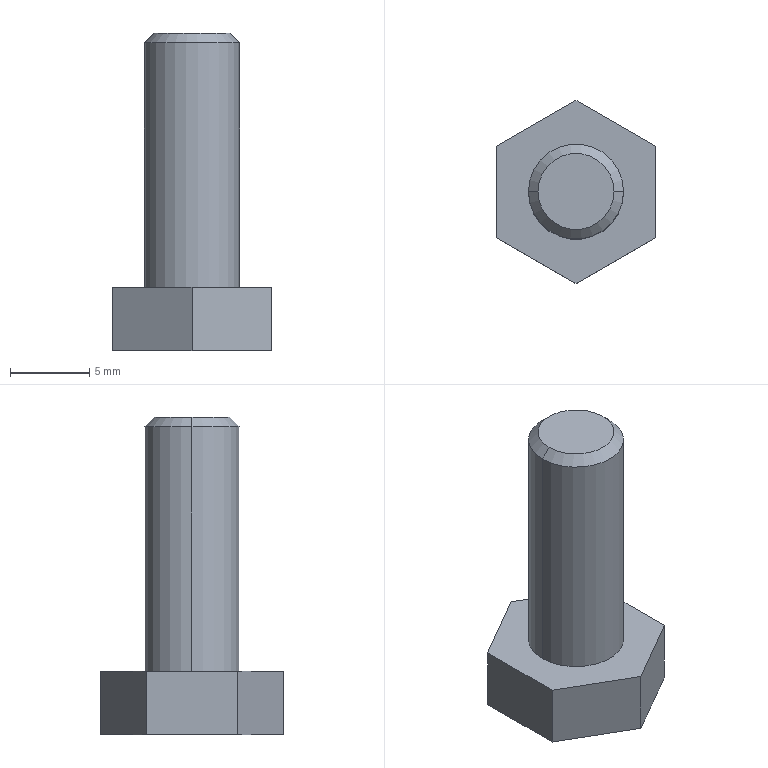Part | SolidWorks | features Chamfer 1, Extrusion 1, ICE 1, RefAxis 1 | 1 solid | 13 faces | box 10 x 11.547 x 20 mm | volume 795.633 mm3 | plane 9 | cone 2 | cylinder 2 | commonest cylinder face diameters 6 x2
STEP:
#1=CARTESIAN_POINT('',(2.4,0.,20.));
#2=VERTEX_POINT('',#1);
#3=CARTESIAN_POINT('',(-2.4,0.,20.));
#4=VERTEX_POINT('',#3);
#5=CARTESIAN_POINT('',(0.,0.,20.));
#6=DIRECTION('',(0.,0.,1.));
#7=DIRECTION('',(1.,0.,0.));
#8=AXIS2_PLACEMENT_3D('',#5,#6,#7);
#9=CIRCLE('',#8,2.4);
#10=EDGE_CURVE('',#2,#4,#9,.T.);
#11=ORIENTED_EDGE('',*,*,#10,.F.);
#12=CARTESIAN_POINT('',(3.,0.,19.4));
#13=VERTEX_POINT('',#12);
#14=CARTESIAN_POINT('',(2.4,0.,20.));
#15=DIRECTION('',(0.7071,0.,-0.7071));
#16=VECTOR('',#15,1000.);
#17=LINE('',#14,#16);
#18=EDGE_CURVE('',#2,#13,#17,.T.);
#19=ORIENTED_EDGE('',*,*,#18,.T.);
#20=CARTESIAN_POINT('',(-3.,0.,19.4));
#21=VERTEX_POINT('',#20);
#22=CARTESIAN_POINT('',(0.,0.,19.4));
#23=DIRECTION('',(0.,0.,-1.));
#24=DIRECTION('',(1.,0.,0.));
#25=AXIS2_PLACEMENT_3D('',#22,#23,#24);
#26=CIRCLE('',#25,3.);
#27=EDGE_CURVE('',#21,#13,#26,.T.);
#28=ORIENTED_EDGE('',*,*,#27,.F.);
#29=CARTESIAN_POINT('',(-2.4,0.,20.));
#30=DIRECTION('',(-0.7071,0.,-0.7071));
#31=VECTOR('',#30,1000.);
#32=LINE('',#29,#31);
#33=EDGE_CURVE('',#4,#21,#32,.T.);
#34=ORIENTED_EDGE('',*,*,#33,.F.);
#35=EDGE_LOOP('',(#11,#19,#28,#34));
#36=FACE_OUTER_BOUND('',#35,.T.);
#37=CARTESIAN_POINT('',(0.,0.,20.));
#38=DIRECTION('',(0.,0.,-1.));
#39=DIRECTION('',(-1.,0.,0.));
#40=AXIS2_PLACEMENT_3D('',#37,#38,#39);
#41=CONICAL_SURFACE('',#40,2.4,0.7854);
#42=ADVANCED_FACE('',(#36),#41,.T.);
#43=ORIENTED_EDGE('',*,*,#27,.T.);
#44=CARTESIAN_POINT('',(3.,0.,4.));
#45=VERTEX_POINT('',#44);
#46=CARTESIAN_POINT('',(3.,0.,20.));
#47=DIRECTION('',(0.,0.,-1.));
#48=VECTOR('',#47,1000.);
#49=LINE('',#46,#48);
#50=EDGE_CURVE('',#13,#45,#49,.T.);
#51=ORIENTED_EDGE('',*,*,#50,.T.);
#52=CARTESIAN_POINT('',(-3.,0.,4.));
#53=VERTEX_POINT('',#52);
#54=CARTESIAN_POINT('',(0.,0.,4.));
#55=DIRECTION('',(0.,0.,1.));
#56=DIRECTION('',(1.,0.,0.));
#57=AXIS2_PLACEMENT_3D('',#54,#55,#56);
#58=CIRCLE('',#57,3.);
#59=EDGE_CURVE('',#45,#53,#58,.T.);
#60=ORIENTED_EDGE('',*,*,#59,.T.);
#61=CARTESIAN_POINT('',(-3.,0.,20.));
#62=DIRECTION('',(0.,0.,-1.));
#63=VECTOR('',#62,1000.);
#64=LINE('',#61,#63);
#65=EDGE_CURVE('',#21,#53,#64,.T.);
#66=ORIENTED_EDGE('',*,*,#65,.F.);
#67=EDGE_LOOP('',(#43,#51,#60,#66));
#68=FACE_OUTER_BOUND('',#67,.T.);
#69=CARTESIAN_POINT('',(0.,0.,20.));
#70=DIRECTION('',(0.,0.,-1.));
#71=DIRECTION('',(-1.,0.,0.));
#72=AXIS2_PLACEMENT_3D('',#69,#70,#71);
#73=CYLINDRICAL_SURFACE('',#72,3.);
#74=ADVANCED_FACE('',(#68),#73,.T.);
#75=CARTESIAN_POINT('',(5.,-2.887,4.));
#76=VERTEX_POINT('',#75);
#77=CARTESIAN_POINT('',(5.,2.887,4.));
#78=VERTEX_POINT('',#77);
#79=CARTESIAN_POINT('',(5.,-2.887,4.));
#80=DIRECTION('',(0.,1.,0.));
#81=VECTOR('',#80,1000.);
#82=LINE('',#79,#81);
#83=EDGE_CURVE('',#76,#78,#82,.T.);
#84=ORIENTED_EDGE('',*,*,#83,.T.);
#85=CARTESIAN_POINT('',(0.,5.774,4.));
#86=VERTEX_POINT('',#85);
#87=CARTESIAN_POINT('',(5.,2.887,4.));
#88=DIRECTION('',(-0.866,0.5,0.));
#89=VECTOR('',#88,1000.);
#90=LINE('',#87,#89);
#91=EDGE_CURVE('',#78,#86,#90,.T.);
#92=ORIENTED_EDGE('',*,*,#91,.T.);
#93=CARTESIAN_POINT('',(-5.,2.887,4.));
#94=VERTEX_POINT('',#93);
#95=CARTESIAN_POINT('',(0.,5.774,4.));
#96=DIRECTION('',(-0.866,-0.5,0.));
#97=VECTOR('',#96,1000.);
#98=LINE('',#95,#97);
#99=EDGE_CURVE('',#86,#94,#98,.T.);
#100=ORIENTED_EDGE('',*,*,#99,.T.);
#101=CARTESIAN_POINT('',(-5.,-2.887,4.));
#102=VERTEX_POINT('',#101);
#103=CARTESIAN_POINT('',(-5.,2.887,4.));
#104=DIRECTION('',(0.,-1.,0.));
#105=VECTOR('',#104,1000.);
#106=LINE('',#103,#105);
#107=EDGE_CURVE('',#94,#102,#106,.T.);
#108=ORIENTED_EDGE('',*,*,#107,.T.);
#109=CARTESIAN_POINT('',(0.,-5.774,4.));
#110=VERTEX_POINT('',#109);
#111=CARTESIAN_POINT('',(-5.,-2.887,4.));
#112=DIRECTION('',(0.866,-0.5,0.));
#113=VECTOR('',#112,1000.);
#114=LINE('',#111,#113);
#115=EDGE_CURVE('',#102,#110,#114,.T.);
#116=ORIENTED_EDGE('',*,*,#115,.T.);
#117=CARTESIAN_POINT('',(0.,-5.774,4.));
#118=DIRECTION('',(0.866,0.5,0.));
#119=VECTOR('',#118,1000.);
#120=LINE('',#117,#119);
#121=EDGE_CURVE('',#110,#76,#120,.T.);
#122=ORIENTED_EDGE('',*,*,#121,.T.);
#123=EDGE_LOOP('',(#84,#92,#100,#108,#116,#122));
#124=FACE_OUTER_BOUND('',#123,.T.);
#125=CARTESIAN_POINT('',(0.,0.,4.));
#126=DIRECTION('',(0.,0.,1.));
#127=DIRECTION('',(1.,0.,0.));
#128=AXIS2_PLACEMENT_3D('',#125,#126,#127);
#129=CIRCLE('',#128,3.);
#130=EDGE_CURVE('',#53,#45,#129,.T.);
#131=ORIENTED_EDGE('',*,*,#130,.F.);
#132=ORIENTED_EDGE('',*,*,#59,.F.);
#133=EDGE_LOOP('',(#131,#132));
#134=FACE_BOUND('',#133,.T.);
#135=CARTESIAN_POINT('',(0.,0.,4.));
#136=DIRECTION('',(0.,0.,1.));
#137=DIRECTION('',(1.,0.,0.));
#138=AXIS2_PLACEMENT_3D('',#135,#136,#137);
#139=PLANE('',#138);
#140=ADVANCED_FACE('',(#124,#134),#139,.T.);
#141=CARTESIAN_POINT('',(5.,-2.887,0.));
#142=VERTEX_POINT('',#141);
#143=CARTESIAN_POINT('',(5.,2.887,0.));
#144=VERTEX_POINT('',#143);
#145=CARTESIAN_POINT('',(5.,-2.887,0.));
#146=DIRECTION('',(0.,1.,0.));
#147=VECTOR('',#146,1000.);
#148=LINE('',#145,#147);
#149=EDGE_CURVE('',#142,#144,#148,.T.);
#150=ORIENTED_EDGE('',*,*,#149,.T.);
#151=CARTESIAN_POINT('',(5.,2.887,4.));
#152=DIRECTION('',(0.,0.,-1.));
#153=VECTOR('',#152,1000.);
#154=LINE('',#151,#153);
#155=EDGE_CURVE('',#78,#144,#154,.T.);
#156=ORIENTED_EDGE('',*,*,#155,.F.);
#157=ORIENTED_EDGE('',*,*,#83,.F.);
#158=CARTESIAN_POINT('',(5.,-2.887,4.));
#159=DIRECTION('',(0.,0.,-1.));
#160=VECTOR('',#159,1000.);
#161=LINE('',#158,#160);
#162=EDGE_CURVE('',#76,#142,#161,.T.);
#163=ORIENTED_EDGE('',*,*,#162,.T.);
#164=EDGE_LOOP('',(#150,#156,#157,#163));
#165=FACE_OUTER_BOUND('',#164,.T.);
#166=CARTESIAN_POINT('',(5.,-2.887,4.));
#167=DIRECTION('',(-1.,0.,0.));
#168=DIRECTION('',(0.,-1.,0.));
#169=AXIS2_PLACEMENT_3D('',#166,#167,#168);
#170=PLANE('',#169);
#171=ADVANCED_FACE('',(#165),#170,.F.);
#172=CARTESIAN_POINT('',(0.,5.774,0.));
#173=VERTEX_POINT('',#172);
#174=CARTESIAN_POINT('',(5.,2.887,0.));
#175=DIRECTION('',(-0.866,0.5,0.));
#176=VECTOR('',#175,1000.);
#177=LINE('',#174,#176);
#178=EDGE_CURVE('',#144,#173,#177,.T.);
#179=ORIENTED_EDGE('',*,*,#178,.T.);
#180=CARTESIAN_POINT('',(0.,5.774,4.));
#181=DIRECTION('',(0.,0.,-1.));
#182=VECTOR('',#181,1000.);
#183=LINE('',#180,#182);
#184=EDGE_CURVE('',#86,#173,#183,.T.);
#185=ORIENTED_EDGE('',*,*,#184,.F.);
#186=ORIENTED_EDGE('',*,*,#91,.F.);
#187=ORIENTED_EDGE('',*,*,#155,.T.);
#188=EDGE_LOOP('',(#179,#185,#186,#187));
#189=FACE_OUTER_BOUND('',#188,.T.);
#190=CARTESIAN_POINT('',(5.,2.887,4.));
#191=DIRECTION('',(-0.5,-0.866,0.));
#192=DIRECTION('',(0.866,-0.5,0.));
#193=AXIS2_PLACEMENT_3D('',#190,#191,#192);
#194=PLANE('',#193);
#195=ADVANCED_FACE('',(#189),#194,.F.);
#196=CARTESIAN_POINT('',(-5.,2.887,0.));
#197=VERTEX_POINT('',#196);
#198=CARTESIAN_POINT('',(0.,5.774,0.));
#199=DIRECTION('',(-0.866,-0.5,0.));
#200=VECTOR('',#199,1000.);
#201=LINE('',#198,#200);
#202=EDGE_CURVE('',#173,#197,#201,.T.);
#203=ORIENTED_EDGE('',*,*,#202,.T.);
#204=CARTESIAN_POINT('',(-5.,2.887,4.));
#205=DIRECTION('',(0.,0.,-1.));
#206=VECTOR('',#205,1000.);
#207=LINE('',#204,#206);
#208=EDGE_CURVE('',#94,#197,#207,.T.);
#209=ORIENTED_EDGE('',*,*,#208,.F.);
#210=ORIENTED_EDGE('',*,*,#99,.F.);
#211=ORIENTED_EDGE('',*,*,#184,.T.);
#212=EDGE_LOOP('',(#203,#209,#210,#211));
#213=FACE_OUTER_BOUND('',#212,.T.);
#214=CARTESIAN_POINT('',(0.,5.774,4.));
#215=DIRECTION('',(0.5,-0.866,0.));
#216=DIRECTION('',(0.866,0.5,0.));
#217=AXIS2_PLACEMENT_3D('',#214,#215,#216);
#218=PLANE('',#217);
#219=ADVANCED_FACE('',(#213),#218,.F.);
#220=CARTESIAN_POINT('',(-5.,-2.887,0.));
#221=VERTEX_POINT('',#220);
#222=CARTESIAN_POINT('',(-5.,2.887,0.));
#223=DIRECTION('',(0.,-1.,0.));
#224=VECTOR('',#223,1000.);
#225=LINE('',#222,#224);
#226=EDGE_CURVE('',#197,#221,#225,.T.);
#227=ORIENTED_EDGE('',*,*,#226,.T.);
#228=CARTESIAN_POINT('',(-5.,-2.887,4.));
#229=DIRECTION('',(0.,0.,-1.));
#230=VECTOR('',#229,1000.);
#231=LINE('',#228,#230);
#232=EDGE_CURVE('',#102,#221,#231,.T.);
#233=ORIENTED_EDGE('',*,*,#232,.F.);
#234=ORIENTED_EDGE('',*,*,#107,.F.);
#235=ORIENTED_EDGE('',*,*,#208,.T.);
#236=EDGE_LOOP('',(#227,#233,#234,#235));
#237=FACE_OUTER_BOUND('',#236,.T.);
#238=CARTESIAN_POINT('',(-5.,2.887,4.));
#239=DIRECTION('',(1.,0.,0.));
#240=DIRECTION('',(0.,1.,0.));
#241=AXIS2_PLACEMENT_3D('',#238,#239,#240);
#242=PLANE('',#241);
#243=ADVANCED_FACE('',(#237),#242,.F.);
#244=CARTESIAN_POINT('',(0.,-5.774,0.));
#245=VERTEX_POINT('',#244);
#246=CARTESIAN_POINT('',(-5.,-2.887,0.));
#247=DIRECTION('',(0.866,-0.5,0.));
#248=VECTOR('',#247,1000.);
#249=LINE('',#246,#248);
#250=EDGE_CURVE('',#221,#245,#249,.T.);
#251=ORIENTED_EDGE('',*,*,#250,.T.);
#252=CARTESIAN_POINT('',(0.,-5.774,4.));
#253=DIRECTION('',(0.,0.,-1.));
#254=VECTOR('',#253,1000.);
#255=LINE('',#252,#254);
#256=EDGE_CURVE('',#110,#245,#255,.T.);
#257=ORIENTED_EDGE('',*,*,#256,.F.);
#258=ORIENTED_EDGE('',*,*,#115,.F.);
#259=ORIENTED_EDGE('',*,*,#232,.T.);
#260=EDGE_LOOP('',(#251,#257,#258,#259));
#261=FACE_OUTER_BOUND('',#260,.T.);
#262=CARTESIAN_POINT('',(-5.,-2.887,4.));
#263=DIRECTION('',(0.5,0.866,0.));
#264=DIRECTION('',(-0.866,0.5,0.));
#265=AXIS2_PLACEMENT_3D('',#262,#263,#264);
#266=PLANE('',#265);
#267=ADVANCED_FACE('',(#261),#266,.F.);
#268=CARTESIAN_POINT('',(0.,-5.774,0.));
#269=DIRECTION('',(0.866,0.5,0.));
#270=VECTOR('',#269,1000.);
#271=LINE('',#268,#270);
#272=EDGE_CURVE('',#245,#142,#271,.T.);
#273=ORIENTED_EDGE('',*,*,#272,.T.);
#274=ORIENTED_EDGE('',*,*,#162,.F.);
#275=ORIENTED_EDGE('',*,*,#121,.F.);
#276=ORIENTED_EDGE('',*,*,#256,.T.);
#277=EDGE_LOOP('',(#273,#274,#275,#276));
#278=FACE_OUTER_BOUND('',#277,.T.);
#279=CARTESIAN_POINT('',(0.,-5.774,4.));
#280=DIRECTION('',(-0.5,0.866,0.));
#281=DIRECTION('',(-0.866,-0.5,0.));
#282=AXIS2_PLACEMENT_3D('',#279,#280,#281);
#283=PLANE('',#282);
#284=ADVANCED_FACE('',(#278),#283,.F.);
#285=ORIENTED_EDGE('',*,*,#149,.F.);
#286=ORIENTED_EDGE('',*,*,#272,.F.);
#287=ORIENTED_EDGE('',*,*,#250,.F.);
#288=ORIENTED_EDGE('',*,*,#226,.F.);
#289=ORIENTED_EDGE('',*,*,#202,.F.);
#290=ORIENTED_EDGE('',*,*,#178,.F.);
#291=EDGE_LOOP('',(#285,#286,#287,#288,#289,#290));
#292=FACE_OUTER_BOUND('',#291,.T.);
#293=CARTESIAN_POINT('',(0.,0.,0.));
#294=DIRECTION('',(0.,0.,1.));
#295=DIRECTION('',(1.,0.,0.));
#296=AXIS2_PLACEMENT_3D('',#293,#294,#295);
#297=PLANE('',#296);
#298=ADVANCED_FACE('',(#292),#297,.F.);
#299=ORIENTED_EDGE('',*,*,#50,.F.);
#300=CARTESIAN_POINT('',(0.,0.,19.4));
#301=DIRECTION('',(0.,0.,-1.));
#302=DIRECTION('',(1.,0.,0.));
#303=AXIS2_PLACEMENT_3D('',#300,#301,#302);
#304=CIRCLE('',#303,3.);
#305=EDGE_CURVE('',#13,#21,#304,.T.);
#306=ORIENTED_EDGE('',*,*,#305,.T.);
#307=ORIENTED_EDGE('',*,*,#65,.T.);
#308=ORIENTED_EDGE('',*,*,#130,.T.);
#309=EDGE_LOOP('',(#299,#306,#307,#308));
#310=FACE_OUTER_BOUND('',#309,.T.);
#311=CARTESIAN_POINT('',(0.,0.,20.));
#312=DIRECTION('',(0.,0.,-1.));
#313=DIRECTION('',(-1.,0.,0.));
#314=AXIS2_PLACEMENT_3D('',#311,#312,#313);
#315=CYLINDRICAL_SURFACE('',#314,3.);
#316=ADVANCED_FACE('',(#310),#315,.T.);
#317=CARTESIAN_POINT('',(0.,0.,20.));
#318=DIRECTION('',(0.,0.,1.));
#319=DIRECTION('',(1.,0.,0.));
#320=AXIS2_PLACEMENT_3D('',#317,#318,#319);
#321=CIRCLE('',#320,2.4);
#322=EDGE_CURVE('',#4,#2,#321,.T.);
#323=ORIENTED_EDGE('',*,*,#322,.T.);
#324=ORIENTED_EDGE('',*,*,#10,.T.);
#325=EDGE_LOOP('',(#323,#324));
#326=FACE_OUTER_BOUND('',#325,.T.);
#327=CARTESIAN_POINT('',(0.,0.,20.));
#328=DIRECTION('',(0.,0.,1.));
#329=DIRECTION('',(1.,0.,0.));
#330=AXIS2_PLACEMENT_3D('',#327,#328,#329);
#331=PLANE('',#330);
#332=ADVANCED_FACE('',(#326),#331,.T.);
#333=ORIENTED_EDGE('',*,*,#18,.F.);
#334=ORIENTED_EDGE('',*,*,#322,.F.);
#335=ORIENTED_EDGE('',*,*,#33,.T.);
#336=ORIENTED_EDGE('',*,*,#305,.F.);
#337=EDGE_LOOP('',(#333,#334,#335,#336));
#338=FACE_OUTER_BOUND('',#337,.T.);
#339=CARTESIAN_POINT('',(0.,0.,20.));
#340=DIRECTION('',(0.,0.,-1.));
#341=DIRECTION('',(-1.,0.,0.));
#342=AXIS2_PLACEMENT_3D('',#339,#340,#341);
#343=CONICAL_SURFACE('',#342,2.4,0.7854);
#344=ADVANCED_FACE('',(#338),#343,.T.);
#345=CLOSED_SHELL('',(#42,#74,#140,#171,#195,#219,#243,#267,#284,#298,#316,#332,#344));
#346=MANIFOLD_SOLID_BREP('',#345);
#347=CARTESIAN_POINT('',(0.,0.,0.));
#348=DIRECTION('',(0.,0.,1.));
#349=DIRECTION('',(1.,0.,0.));
#350=AXIS2_PLACEMENT_3D('',#347,#348,#349);
#351=(LENGTH_UNIT()NAMED_UNIT(*)SI_UNIT(.MILLI.,.METRE.));
#352=UNCERTAINTY_MEASURE_WITH_UNIT(LENGTH_MEASURE(0.00001),#351,'','');
#353=(NAMED_UNIT(*)PLANE_ANGLE_UNIT()SI_UNIT($,.RADIAN.));
#354=(NAMED_UNIT(*)SI_UNIT($,.STERADIAN.)SOLID_ANGLE_UNIT());
#355=(GEOMETRIC_REPRESENTATION_CONTEXT(3)GLOBAL_UNCERTAINTY_ASSIGNED_CONTEXT((#352))GLOBAL_UNIT_ASSIGNED_CONTEXT((#351,#353,#354))REPRESENTATION_CONTEXT('',''));
#356=ADVANCED_BREP_SHAPE_REPRESENTATION('',(#346,#350),#355);